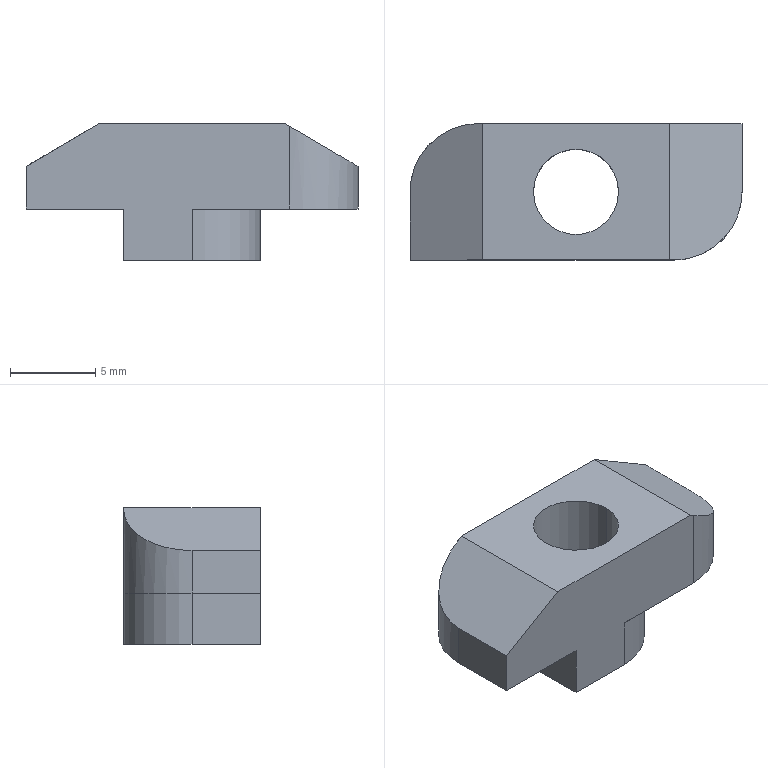Part | NX | features BREP 1 | 1 solid | 18 faces | box 19.5 x 8 x 8 mm | volume 688.541 mm3 | plane 12 | cylinder 6 | commonest cylinder face diameters 8 x4 5 x2
STEP:
#1=CARTESIAN_POINT('',(-2.5,0.,-8.));
#2=VERTEX_POINT('',#1);
#3=CARTESIAN_POINT('',(2.5,0.,-8.));
#4=VERTEX_POINT('',#3);
#5=CARTESIAN_POINT('',(0.,0.,-8.));
#6=DIRECTION('',(0.,0.,-1.));
#7=DIRECTION('',(-1.,0.,0.));
#8=AXIS2_PLACEMENT_3D('',#5,#6,#7);
#9=CIRCLE('',#8,2.5);
#10=EDGE_CURVE('',#2,#4,#9,.T.);
#11=ORIENTED_EDGE('',*,*,#10,.T.);
#12=CARTESIAN_POINT('',(2.5,0.,0.));
#13=VERTEX_POINT('',#12);
#14=CARTESIAN_POINT('',(2.5,0.,0.));
#15=DIRECTION('',(0.,0.,1.));
#16=VECTOR('',#15,1000.);
#17=LINE('',#14,#16);
#18=EDGE_CURVE('',#4,#13,#17,.T.);
#19=ORIENTED_EDGE('',*,*,#18,.T.);
#20=CARTESIAN_POINT('',(-2.5,0.,0.));
#21=VERTEX_POINT('',#20);
#22=CARTESIAN_POINT('',(0.,0.,0.));
#23=DIRECTION('',(0.,0.,-1.));
#24=DIRECTION('',(-1.,0.,0.));
#25=AXIS2_PLACEMENT_3D('',#22,#23,#24);
#26=CIRCLE('',#25,2.5);
#27=EDGE_CURVE('',#21,#13,#26,.T.);
#28=ORIENTED_EDGE('',*,*,#27,.F.);
#29=CARTESIAN_POINT('',(-2.5,0.,0.));
#30=DIRECTION('',(0.,0.,1.));
#31=VECTOR('',#30,1000.);
#32=LINE('',#29,#31);
#33=EDGE_CURVE('',#2,#21,#32,.T.);
#34=ORIENTED_EDGE('',*,*,#33,.F.);
#35=EDGE_LOOP('',(#11,#19,#28,#34));
#36=FACE_BOUND('',#35,.T.);
#37=CARTESIAN_POINT('',(0.,0.,0.));
#38=DIRECTION('',(0.,0.,1.));
#39=DIRECTION('',(-1.,0.,0.));
#40=AXIS2_PLACEMENT_3D('',#37,#38,#39);
#41=CYLINDRICAL_SURFACE('',#40,2.5);
#42=ADVANCED_FACE('',(#36),#41,.F.);
#43=CARTESIAN_POINT('',(0.,-4.,-5.));
#44=VERTEX_POINT('',#43);
#45=CARTESIAN_POINT('',(5.75,-4.,-5.));
#46=VERTEX_POINT('',#45);
#47=CARTESIAN_POINT('',(-9.75,-4.,-5.));
#48=DIRECTION('',(1.,0.,0.));
#49=VECTOR('',#48,1000.);
#50=LINE('',#47,#49);
#51=EDGE_CURVE('',#44,#46,#50,.T.);
#52=ORIENTED_EDGE('',*,*,#51,.F.);
#53=CARTESIAN_POINT('',(4.,0.,-5.));
#54=VERTEX_POINT('',#53);
#55=CARTESIAN_POINT('',(0.,0.,-5.));
#56=DIRECTION('',(0.,0.,-1.));
#57=DIRECTION('',(1.,0.,0.));
#58=AXIS2_PLACEMENT_3D('',#55,#56,#57);
#59=CIRCLE('',#58,4.);
#60=EDGE_CURVE('',#54,#44,#59,.T.);
#61=ORIENTED_EDGE('',*,*,#60,.F.);
#62=CARTESIAN_POINT('',(4.,4.,-5.));
#63=VERTEX_POINT('',#62);
#64=CARTESIAN_POINT('',(4.,-4.,-5.));
#65=DIRECTION('',(0.,1.,0.));
#66=VECTOR('',#65,1000.);
#67=LINE('',#64,#66);
#68=EDGE_CURVE('',#54,#63,#67,.T.);
#69=ORIENTED_EDGE('',*,*,#68,.T.);
#70=CARTESIAN_POINT('',(9.75,4.,-5.));
#71=VERTEX_POINT('',#70);
#72=CARTESIAN_POINT('',(-9.75,4.,-5.));
#73=DIRECTION('',(-1.,0.,0.));
#74=VECTOR('',#73,1000.);
#75=LINE('',#72,#74);
#76=EDGE_CURVE('',#71,#63,#75,.T.);
#77=ORIENTED_EDGE('',*,*,#76,.F.);
#78=CARTESIAN_POINT('',(9.75,0.,-5.));
#79=VERTEX_POINT('',#78);
#80=CARTESIAN_POINT('',(9.75,4.,-5.));
#81=DIRECTION('',(0.,1.,0.));
#82=VECTOR('',#81,1000.);
#83=LINE('',#80,#82);
#84=EDGE_CURVE('',#79,#71,#83,.T.);
#85=ORIENTED_EDGE('',*,*,#84,.F.);
#86=CARTESIAN_POINT('',(5.75,0.,-5.));
#87=DIRECTION('',(0.,0.,1.));
#88=DIRECTION('',(1.,0.,0.));
#89=AXIS2_PLACEMENT_3D('',#86,#87,#88);
#90=CIRCLE('',#89,4.);
#91=EDGE_CURVE('',#46,#79,#90,.T.);
#92=ORIENTED_EDGE('',*,*,#91,.F.);
#93=EDGE_LOOP('',(#52,#61,#69,#77,#85,#92));
#94=FACE_BOUND('',#93,.T.);
#95=CARTESIAN_POINT('',(0.,0.,-5.));
#96=DIRECTION('',(0.,0.,-1.));
#97=DIRECTION('',(0.,-1.,0.));
#98=AXIS2_PLACEMENT_3D('',#95,#96,#97);
#99=PLANE('',#98);
#100=ADVANCED_FACE('',(#94),#99,.T.);
#101=ORIENTED_EDGE('',*,*,#84,.T.);
#102=CARTESIAN_POINT('',(9.75,4.,-2.5));
#103=VERTEX_POINT('',#102);
#104=CARTESIAN_POINT('',(9.75,4.,-5.));
#105=DIRECTION('',(0.,0.,1.));
#106=VECTOR('',#105,1000.);
#107=LINE('',#104,#106);
#108=EDGE_CURVE('',#71,#103,#107,.T.);
#109=ORIENTED_EDGE('',*,*,#108,.T.);
#110=CARTESIAN_POINT('',(9.75,0.,-2.5));
#111=VERTEX_POINT('',#110);
#112=CARTESIAN_POINT('',(9.75,4.,-2.5));
#113=DIRECTION('',(0.,1.,0.));
#114=VECTOR('',#113,1000.);
#115=LINE('',#112,#114);
#116=EDGE_CURVE('',#111,#103,#115,.T.);
#117=ORIENTED_EDGE('',*,*,#116,.F.);
#118=CARTESIAN_POINT('',(9.75,0.,-5.));
#119=DIRECTION('',(0.,0.,1.));
#120=VECTOR('',#119,1000.);
#121=LINE('',#118,#120);
#122=EDGE_CURVE('',#79,#111,#121,.T.);
#123=ORIENTED_EDGE('',*,*,#122,.F.);
#124=EDGE_LOOP('',(#101,#109,#117,#123));
#125=FACE_BOUND('',#124,.T.);
#126=CARTESIAN_POINT('',(9.75,4.,-5.));
#127=DIRECTION('',(-1.,0.,0.));
#128=DIRECTION('',(0.,0.,1.));
#129=AXIS2_PLACEMENT_3D('',#126,#127,#128);
#130=PLANE('',#129);
#131=ADVANCED_FACE('',(#125),#130,.F.);
#132=CARTESIAN_POINT('',(-5.5,4.,0.));
#133=VERTEX_POINT('',#132);
#134=CARTESIAN_POINT('',(-5.75,4.,-0.1471));
#135=VERTEX_POINT('',#134);
#136=CARTESIAN_POINT('',(-9.75,4.,-2.5));
#137=DIRECTION('',(-0.8619,0.,-0.507));
#138=VECTOR('',#137,1000.);
#139=LINE('',#136,#138);
#140=EDGE_CURVE('',#133,#135,#139,.T.);
#141=ORIENTED_EDGE('',*,*,#140,.F.);
#142=CARTESIAN_POINT('',(5.5,4.,0.));
#143=VERTEX_POINT('',#142);
#144=CARTESIAN_POINT('',(-9.75,4.,0.));
#145=DIRECTION('',(-1.,0.,0.));
#146=VECTOR('',#145,1000.);
#147=LINE('',#144,#146);
#148=EDGE_CURVE('',#143,#133,#147,.T.);
#149=ORIENTED_EDGE('',*,*,#148,.F.);
#150=CARTESIAN_POINT('',(9.75,4.,-2.5));
#151=DIRECTION('',(-0.8619,0.,0.507));
#152=VECTOR('',#151,1000.);
#153=LINE('',#150,#152);
#154=EDGE_CURVE('',#103,#143,#153,.T.);
#155=ORIENTED_EDGE('',*,*,#154,.F.);
#156=ORIENTED_EDGE('',*,*,#108,.F.);
#157=ORIENTED_EDGE('',*,*,#76,.T.);
#158=CARTESIAN_POINT('',(4.,4.,-8.));
#159=VERTEX_POINT('',#158);
#160=CARTESIAN_POINT('',(4.,4.,-8.));
#161=DIRECTION('',(0.,0.,1.));
#162=VECTOR('',#161,1000.);
#163=LINE('',#160,#162);
#164=EDGE_CURVE('',#159,#63,#163,.T.);
#165=ORIENTED_EDGE('',*,*,#164,.F.);
#166=CARTESIAN_POINT('',(0.,4.,-8.));
#167=VERTEX_POINT('',#166);
#168=CARTESIAN_POINT('',(-4.,4.,-8.));
#169=DIRECTION('',(-1.,0.,0.));
#170=VECTOR('',#169,1000.);
#171=LINE('',#168,#170);
#172=EDGE_CURVE('',#159,#167,#171,.T.);
#173=ORIENTED_EDGE('',*,*,#172,.T.);
#174=CARTESIAN_POINT('',(0.,4.,-5.));
#175=VERTEX_POINT('',#174);
#176=CARTESIAN_POINT('',(0.,4.,-5.));
#177=DIRECTION('',(0.,0.,-1.));
#178=VECTOR('',#177,1000.);
#179=LINE('',#176,#178);
#180=EDGE_CURVE('',#175,#167,#179,.T.);
#181=ORIENTED_EDGE('',*,*,#180,.F.);
#182=CARTESIAN_POINT('',(-5.75,4.,-5.));
#183=VERTEX_POINT('',#182);
#184=CARTESIAN_POINT('',(-9.75,4.,-5.));
#185=DIRECTION('',(-1.,0.,0.));
#186=VECTOR('',#185,1000.);
#187=LINE('',#184,#186);
#188=EDGE_CURVE('',#175,#183,#187,.T.);
#189=ORIENTED_EDGE('',*,*,#188,.T.);
#190=CARTESIAN_POINT('',(-5.75,4.,-5.));
#191=DIRECTION('',(0.,0.,-1.));
#192=VECTOR('',#191,1000.);
#193=LINE('',#190,#192);
#194=EDGE_CURVE('',#135,#183,#193,.T.);
#195=ORIENTED_EDGE('',*,*,#194,.F.);
#196=EDGE_LOOP('',(#141,#149,#155,#156,#157,#165,#173,#181,#189,#195));
#197=FACE_BOUND('',#196,.T.);
#198=CARTESIAN_POINT('',(-9.75,4.,-5.));
#199=DIRECTION('',(0.,-1.,0.));
#200=DIRECTION('',(0.,0.,-1.));
#201=AXIS2_PLACEMENT_3D('',#198,#199,#200);
#202=PLANE('',#201);
#203=ADVANCED_FACE('',(#197),#202,.F.);
#204=CARTESIAN_POINT('',(-9.75,0.,-5.));
#205=VERTEX_POINT('',#204);
#206=CARTESIAN_POINT('',(-9.75,-4.,-5.));
#207=VERTEX_POINT('',#206);
#208=CARTESIAN_POINT('',(-9.75,4.,-5.));
#209=DIRECTION('',(0.,-1.,0.));
#210=VECTOR('',#209,1000.);
#211=LINE('',#208,#210);
#212=EDGE_CURVE('',#205,#207,#211,.T.);
#213=ORIENTED_EDGE('',*,*,#212,.T.);
#214=CARTESIAN_POINT('',(-9.75,-4.,-2.5));
#215=VERTEX_POINT('',#214);
#216=CARTESIAN_POINT('',(-9.75,-4.,-5.));
#217=DIRECTION('',(0.,0.,1.));
#218=VECTOR('',#217,1000.);
#219=LINE('',#216,#218);
#220=EDGE_CURVE('',#207,#215,#219,.T.);
#221=ORIENTED_EDGE('',*,*,#220,.T.);
#222=CARTESIAN_POINT('',(-9.75,0.,-2.5));
#223=VERTEX_POINT('',#222);
#224=CARTESIAN_POINT('',(-9.75,4.,-2.5));
#225=DIRECTION('',(0.,-1.,0.));
#226=VECTOR('',#225,1000.);
#227=LINE('',#224,#226);
#228=EDGE_CURVE('',#223,#215,#227,.T.);
#229=ORIENTED_EDGE('',*,*,#228,.F.);
#230=CARTESIAN_POINT('',(-9.75,0.,-5.));
#231=DIRECTION('',(0.,0.,1.));
#232=VECTOR('',#231,1000.);
#233=LINE('',#230,#232);
#234=EDGE_CURVE('',#205,#223,#233,.T.);
#235=ORIENTED_EDGE('',*,*,#234,.F.);
#236=EDGE_LOOP('',(#213,#221,#229,#235));
#237=FACE_BOUND('',#236,.T.);
#238=CARTESIAN_POINT('',(-9.75,4.,-5.));
#239=DIRECTION('',(1.,0.,0.));
#240=DIRECTION('',(0.,1.,0.));
#241=AXIS2_PLACEMENT_3D('',#238,#239,#240);
#242=PLANE('',#241);
#243=ADVANCED_FACE('',(#237),#242,.F.);
#244=CARTESIAN_POINT('',(5.5,-4.,0.));
#245=VERTEX_POINT('',#244);
#246=CARTESIAN_POINT('',(5.75,-4.,-0.1471));
#247=VERTEX_POINT('',#246);
#248=CARTESIAN_POINT('',(9.75,-4.,-2.5));
#249=DIRECTION('',(0.8619,0.,-0.507));
#250=VECTOR('',#249,1000.);
#251=LINE('',#248,#250);
#252=EDGE_CURVE('',#245,#247,#251,.T.);
#253=ORIENTED_EDGE('',*,*,#252,.F.);
#254=CARTESIAN_POINT('',(-5.5,-4.,0.));
#255=VERTEX_POINT('',#254);
#256=CARTESIAN_POINT('',(-9.75,-4.,0.));
#257=DIRECTION('',(1.,0.,0.));
#258=VECTOR('',#257,1000.);
#259=LINE('',#256,#258);
#260=EDGE_CURVE('',#255,#245,#259,.T.);
#261=ORIENTED_EDGE('',*,*,#260,.F.);
#262=CARTESIAN_POINT('',(-9.75,-4.,-2.5));
#263=DIRECTION('',(0.8619,0.,0.507));
#264=VECTOR('',#263,1000.);
#265=LINE('',#262,#264);
#266=EDGE_CURVE('',#215,#255,#265,.T.);
#267=ORIENTED_EDGE('',*,*,#266,.F.);
#268=ORIENTED_EDGE('',*,*,#220,.F.);
#269=CARTESIAN_POINT('',(-4.,-4.,-5.));
#270=VERTEX_POINT('',#269);
#271=CARTESIAN_POINT('',(-9.75,-4.,-5.));
#272=DIRECTION('',(1.,0.,0.));
#273=VECTOR('',#272,1000.);
#274=LINE('',#271,#273);
#275=EDGE_CURVE('',#207,#270,#274,.T.);
#276=ORIENTED_EDGE('',*,*,#275,.T.);
#277=CARTESIAN_POINT('',(-4.,-4.,-8.));
#278=VERTEX_POINT('',#277);
#279=CARTESIAN_POINT('',(-4.,-4.,-8.));
#280=DIRECTION('',(0.,0.,1.));
#281=VECTOR('',#280,1000.);
#282=LINE('',#279,#281);
#283=EDGE_CURVE('',#278,#270,#282,.T.);
#284=ORIENTED_EDGE('',*,*,#283,.F.);
#285=CARTESIAN_POINT('',(0.,-4.,-8.));
#286=VERTEX_POINT('',#285);
#287=CARTESIAN_POINT('',(-4.,-4.,-8.));
#288=DIRECTION('',(1.,0.,0.));
#289=VECTOR('',#288,1000.);
#290=LINE('',#287,#289);
#291=EDGE_CURVE('',#278,#286,#290,.T.);
#292=ORIENTED_EDGE('',*,*,#291,.T.);
#293=CARTESIAN_POINT('',(0.,-4.,-5.));
#294=DIRECTION('',(0.,0.,-1.));
#295=VECTOR('',#294,1000.);
#296=LINE('',#293,#295);
#297=EDGE_CURVE('',#44,#286,#296,.T.);
#298=ORIENTED_EDGE('',*,*,#297,.F.);
#299=ORIENTED_EDGE('',*,*,#51,.T.);
#300=CARTESIAN_POINT('',(5.75,-4.,-5.));
#301=DIRECTION('',(0.,0.,-1.));
#302=VECTOR('',#301,1000.);
#303=LINE('',#300,#302);
#304=EDGE_CURVE('',#247,#46,#303,.T.);
#305=ORIENTED_EDGE('',*,*,#304,.F.);
#306=EDGE_LOOP('',(#253,#261,#267,#268,#276,#284,#292,#298,#299,#305));
#307=FACE_BOUND('',#306,.T.);
#308=CARTESIAN_POINT('',(-9.75,-4.,-5.));
#309=DIRECTION('',(0.,1.,0.));
#310=DIRECTION('',(1.,0.,0.));
#311=AXIS2_PLACEMENT_3D('',#308,#309,#310);
#312=PLANE('',#311);
#313=ADVANCED_FACE('',(#307),#312,.F.);
#314=ORIENTED_EDGE('',*,*,#188,.F.);
#315=CARTESIAN_POINT('',(-4.,0.,-5.));
#316=VERTEX_POINT('',#315);
#317=CARTESIAN_POINT('',(0.,0.,-5.));
#318=DIRECTION('',(0.,0.,-1.));
#319=DIRECTION('',(1.,0.,0.));
#320=AXIS2_PLACEMENT_3D('',#317,#318,#319);
#321=CIRCLE('',#320,4.);
#322=EDGE_CURVE('',#316,#175,#321,.T.);
#323=ORIENTED_EDGE('',*,*,#322,.F.);
#324=CARTESIAN_POINT('',(-4.,-4.,-5.));
#325=DIRECTION('',(0.,-1.,0.));
#326=VECTOR('',#325,1000.);
#327=LINE('',#324,#326);
#328=EDGE_CURVE('',#316,#270,#327,.T.);
#329=ORIENTED_EDGE('',*,*,#328,.T.);
#330=ORIENTED_EDGE('',*,*,#275,.F.);
#331=ORIENTED_EDGE('',*,*,#212,.F.);
#332=CARTESIAN_POINT('',(-5.75,0.,-5.));
#333=DIRECTION('',(0.,0.,1.));
#334=DIRECTION('',(1.,0.,0.));
#335=AXIS2_PLACEMENT_3D('',#332,#333,#334);
#336=CIRCLE('',#335,4.);
#337=EDGE_CURVE('',#183,#205,#336,.T.);
#338=ORIENTED_EDGE('',*,*,#337,.F.);
#339=EDGE_LOOP('',(#314,#323,#329,#330,#331,#338));
#340=FACE_BOUND('',#339,.T.);
#341=CARTESIAN_POINT('',(0.,0.,-5.));
#342=DIRECTION('',(0.,0.,-1.));
#343=DIRECTION('',(0.,-1.,0.));
#344=AXIS2_PLACEMENT_3D('',#341,#342,#343);
#345=PLANE('',#344);
#346=ADVANCED_FACE('',(#340),#345,.T.);
#347=ORIENTED_EDGE('',*,*,#148,.T.);
#348=CARTESIAN_POINT('',(-5.5,0.,0.));
#349=DIRECTION('',(0.,1.,0.));
#350=VECTOR('',#349,1000.);
#351=LINE('',#348,#350);
#352=EDGE_CURVE('',#255,#133,#351,.T.);
#353=ORIENTED_EDGE('',*,*,#352,.F.);
#354=ORIENTED_EDGE('',*,*,#260,.T.);
#355=CARTESIAN_POINT('',(5.5,0.,0.));
#356=DIRECTION('',(0.,-1.,0.));
#357=VECTOR('',#356,1000.);
#358=LINE('',#355,#357);
#359=EDGE_CURVE('',#143,#245,#358,.T.);
#360=ORIENTED_EDGE('',*,*,#359,.F.);
#361=EDGE_LOOP('',(#347,#353,#354,#360));
#362=FACE_BOUND('',#361,.T.);
#363=ORIENTED_EDGE('',*,*,#27,.T.);
#364=CARTESIAN_POINT('',(0.,0.,0.));
#365=DIRECTION('',(0.,0.,-1.));
#366=DIRECTION('',(-1.,0.,0.));
#367=AXIS2_PLACEMENT_3D('',#364,#365,#366);
#368=CIRCLE('',#367,2.5);
#369=EDGE_CURVE('',#13,#21,#368,.T.);
#370=ORIENTED_EDGE('',*,*,#369,.T.);
#371=EDGE_LOOP('',(#363,#370));
#372=FACE_BOUND('',#371,.T.);
#373=CARTESIAN_POINT('',(0.,0.,0.));
#374=DIRECTION('',(0.,0.,-1.));
#375=DIRECTION('',(0.,-1.,0.));
#376=AXIS2_PLACEMENT_3D('',#373,#374,#375);
#377=PLANE('',#376);
#378=ADVANCED_FACE('',(#362,#372),#377,.F.);
#379=CARTESIAN_POINT('',(4.,0.,-8.));
#380=VERTEX_POINT('',#379);
#381=CARTESIAN_POINT('',(4.,-4.,-8.));
#382=DIRECTION('',(0.,1.,0.));
#383=VECTOR('',#382,1000.);
#384=LINE('',#381,#383);
#385=EDGE_CURVE('',#380,#159,#384,.T.);
#386=ORIENTED_EDGE('',*,*,#385,.T.);
#387=ORIENTED_EDGE('',*,*,#164,.T.);
#388=ORIENTED_EDGE('',*,*,#68,.F.);
#389=CARTESIAN_POINT('',(4.,0.,-8.));
#390=DIRECTION('',(0.,0.,1.));
#391=VECTOR('',#390,1000.);
#392=LINE('',#389,#391);
#393=EDGE_CURVE('',#380,#54,#392,.T.);
#394=ORIENTED_EDGE('',*,*,#393,.F.);
#395=EDGE_LOOP('',(#386,#387,#388,#394));
#396=FACE_BOUND('',#395,.T.);
#397=CARTESIAN_POINT('',(4.,-4.,-8.));
#398=DIRECTION('',(-1.,0.,0.));
#399=DIRECTION('',(0.,0.,1.));
#400=AXIS2_PLACEMENT_3D('',#397,#398,#399);
#401=PLANE('',#400);
#402=ADVANCED_FACE('',(#396),#401,.F.);
#403=CARTESIAN_POINT('',(-4.,0.,-8.));
#404=VERTEX_POINT('',#403);
#405=CARTESIAN_POINT('',(-4.,-4.,-8.));
#406=DIRECTION('',(0.,-1.,0.));
#407=VECTOR('',#406,1000.);
#408=LINE('',#405,#407);
#409=EDGE_CURVE('',#404,#278,#408,.T.);
#410=ORIENTED_EDGE('',*,*,#409,.T.);
#411=ORIENTED_EDGE('',*,*,#283,.T.);
#412=ORIENTED_EDGE('',*,*,#328,.F.);
#413=CARTESIAN_POINT('',(-4.,0.,-8.));
#414=DIRECTION('',(0.,0.,1.));
#415=VECTOR('',#414,1000.);
#416=LINE('',#413,#415);
#417=EDGE_CURVE('',#404,#316,#416,.T.);
#418=ORIENTED_EDGE('',*,*,#417,.F.);
#419=EDGE_LOOP('',(#410,#411,#412,#418));
#420=FACE_BOUND('',#419,.T.);
#421=CARTESIAN_POINT('',(-4.,-4.,-8.));
#422=DIRECTION('',(1.,0.,0.));
#423=DIRECTION('',(0.,1.,0.));
#424=AXIS2_PLACEMENT_3D('',#421,#422,#423);
#425=PLANE('',#424);
#426=ADVANCED_FACE('',(#420),#425,.F.);
#427=ORIENTED_EDGE('',*,*,#291,.F.);
#428=ORIENTED_EDGE('',*,*,#409,.F.);
#429=CARTESIAN_POINT('',(0.,0.,-8.));
#430=DIRECTION('',(0.,0.,1.));
#431=DIRECTION('',(-1.,0.,0.));
#432=AXIS2_PLACEMENT_3D('',#429,#430,#431);
#433=CIRCLE('',#432,4.);
#434=EDGE_CURVE('',#167,#404,#433,.T.);
#435=ORIENTED_EDGE('',*,*,#434,.F.);
#436=ORIENTED_EDGE('',*,*,#172,.F.);
#437=ORIENTED_EDGE('',*,*,#385,.F.);
#438=CARTESIAN_POINT('',(0.,0.,-8.));
#439=DIRECTION('',(0.,0.,1.));
#440=DIRECTION('',(-1.,0.,0.));
#441=AXIS2_PLACEMENT_3D('',#438,#439,#440);
#442=CIRCLE('',#441,4.);
#443=EDGE_CURVE('',#286,#380,#442,.T.);
#444=ORIENTED_EDGE('',*,*,#443,.F.);
#445=EDGE_LOOP('',(#427,#428,#435,#436,#437,#444));
#446=FACE_BOUND('',#445,.T.);
#447=ORIENTED_EDGE('',*,*,#10,.F.);
#448=CARTESIAN_POINT('',(0.,0.,-8.));
#449=DIRECTION('',(0.,0.,-1.));
#450=DIRECTION('',(-1.,0.,0.));
#451=AXIS2_PLACEMENT_3D('',#448,#449,#450);
#452=CIRCLE('',#451,2.5);
#453=EDGE_CURVE('',#4,#2,#452,.T.);
#454=ORIENTED_EDGE('',*,*,#453,.F.);
#455=EDGE_LOOP('',(#447,#454));
#456=FACE_BOUND('',#455,.T.);
#457=CARTESIAN_POINT('',(0.,0.,-8.));
#458=DIRECTION('',(0.,0.,1.));
#459=DIRECTION('',(1.,0.,0.));
#460=AXIS2_PLACEMENT_3D('',#457,#458,#459);
#461=PLANE('',#460);
#462=ADVANCED_FACE('',(#446,#456),#461,.F.);
#463=ORIENTED_EDGE('',*,*,#18,.F.);
#464=ORIENTED_EDGE('',*,*,#453,.T.);
#465=ORIENTED_EDGE('',*,*,#33,.T.);
#466=ORIENTED_EDGE('',*,*,#369,.F.);
#467=EDGE_LOOP('',(#463,#464,#465,#466));
#468=FACE_BOUND('',#467,.T.);
#469=CARTESIAN_POINT('',(0.,0.,0.));
#470=DIRECTION('',(0.,0.,1.));
#471=DIRECTION('',(-1.,0.,0.));
#472=AXIS2_PLACEMENT_3D('',#469,#470,#471);
#473=CYLINDRICAL_SURFACE('',#472,2.5);
#474=ADVANCED_FACE('',(#468),#473,.F.);
#475=ORIENTED_EDGE('',*,*,#116,.T.);
#476=ORIENTED_EDGE('',*,*,#154,.T.);
#477=ORIENTED_EDGE('',*,*,#359,.T.);
#478=ORIENTED_EDGE('',*,*,#252,.T.);
#479=CARTESIAN_POINT('',(9.75,0.,-2.5));
#480=CARTESIAN_POINT('',(9.75,-2.343,-2.5));
#481=CARTESIAN_POINT('',(8.093,-4.,-1.525));
#482=CARTESIAN_POINT('',(5.75,-4.,-0.1471));
#483=(BOUNDED_CURVE()B_SPLINE_CURVE(3,(#479,#480,#481,#482),.UNSPECIFIED.,.F.,.F.)B_SPLINE_CURVE_WITH_KNOTS((4,4),(3.142,4.712),.UNSPECIFIED.)CURVE()GEOMETRIC_REPRESENTATION_ITEM()RATIONAL_B_SPLINE_CURVE((1.,0.8047,0.8047,1.))REPRESENTATION_ITEM(''));
#484=EDGE_CURVE('',#111,#247,#483,.T.);
#485=ORIENTED_EDGE('',*,*,#484,.F.);
#486=EDGE_LOOP('',(#475,#476,#477,#478,#485));
#487=FACE_BOUND('',#486,.T.);
#488=CARTESIAN_POINT('',(9.75,4.,-2.5));
#489=DIRECTION('',(-0.507,0.,-0.8619));
#490=DIRECTION('',(-0.8619,0.,0.507));
#491=AXIS2_PLACEMENT_3D('',#488,#489,#490);
#492=PLANE('',#491);
#493=ADVANCED_FACE('',(#487),#492,.F.);
#494=ORIENTED_EDGE('',*,*,#228,.T.);
#495=ORIENTED_EDGE('',*,*,#266,.T.);
#496=ORIENTED_EDGE('',*,*,#352,.T.);
#497=ORIENTED_EDGE('',*,*,#140,.T.);
#498=CARTESIAN_POINT('',(-9.75,0.,-2.5));
#499=CARTESIAN_POINT('',(-9.75,2.343,-2.5));
#500=CARTESIAN_POINT('',(-8.093,4.,-1.525));
#501=CARTESIAN_POINT('',(-5.75,4.,-0.1471));
#502=(BOUNDED_CURVE()B_SPLINE_CURVE(3,(#498,#499,#500,#501),.UNSPECIFIED.,.F.,.F.)B_SPLINE_CURVE_WITH_KNOTS((4,4),(3.142,4.712),.UNSPECIFIED.)CURVE()GEOMETRIC_REPRESENTATION_ITEM()RATIONAL_B_SPLINE_CURVE((1.,0.8047,0.8047,1.))REPRESENTATION_ITEM(''));
#503=EDGE_CURVE('',#223,#135,#502,.T.);
#504=ORIENTED_EDGE('',*,*,#503,.F.);
#505=EDGE_LOOP('',(#494,#495,#496,#497,#504));
#506=FACE_BOUND('',#505,.T.);
#507=CARTESIAN_POINT('',(-9.75,4.,-2.5));
#508=DIRECTION('',(0.507,0.,-0.8619));
#509=DIRECTION('',(0.,-1.,0.));
#510=AXIS2_PLACEMENT_3D('',#507,#508,#509);
#511=PLANE('',#510);
#512=ADVANCED_FACE('',(#506),#511,.F.);
#513=ORIENTED_EDGE('',*,*,#91,.T.);
#514=ORIENTED_EDGE('',*,*,#122,.T.);
#515=ORIENTED_EDGE('',*,*,#484,.T.);
#516=ORIENTED_EDGE('',*,*,#304,.T.);
#517=EDGE_LOOP('',(#513,#514,#515,#516));
#518=FACE_BOUND('',#517,.T.);
#519=CARTESIAN_POINT('',(5.75,0.,-5.));
#520=DIRECTION('',(0.,0.,1.));
#521=DIRECTION('',(-1.,0.,0.));
#522=AXIS2_PLACEMENT_3D('',#519,#520,#521);
#523=CYLINDRICAL_SURFACE('',#522,4.);
#524=ADVANCED_FACE('',(#518),#523,.T.);
#525=ORIENTED_EDGE('',*,*,#337,.T.);
#526=ORIENTED_EDGE('',*,*,#234,.T.);
#527=ORIENTED_EDGE('',*,*,#503,.T.);
#528=ORIENTED_EDGE('',*,*,#194,.T.);
#529=EDGE_LOOP('',(#525,#526,#527,#528));
#530=FACE_BOUND('',#529,.T.);
#531=CARTESIAN_POINT('',(-5.75,0.,-5.));
#532=DIRECTION('',(0.,0.,1.));
#533=DIRECTION('',(-1.,0.,0.));
#534=AXIS2_PLACEMENT_3D('',#531,#532,#533);
#535=CYLINDRICAL_SURFACE('',#534,4.);
#536=ADVANCED_FACE('',(#530),#535,.T.);
#537=ORIENTED_EDGE('',*,*,#443,.T.);
#538=ORIENTED_EDGE('',*,*,#393,.T.);
#539=ORIENTED_EDGE('',*,*,#60,.T.);
#540=ORIENTED_EDGE('',*,*,#297,.T.);
#541=EDGE_LOOP('',(#537,#538,#539,#540));
#542=FACE_BOUND('',#541,.T.);
#543=CARTESIAN_POINT('',(0.,0.,-8.));
#544=DIRECTION('',(0.,0.,1.));
#545=DIRECTION('',(-1.,0.,0.));
#546=AXIS2_PLACEMENT_3D('',#543,#544,#545);
#547=CYLINDRICAL_SURFACE('',#546,4.);
#548=ADVANCED_FACE('',(#542),#547,.T.);
#549=ORIENTED_EDGE('',*,*,#434,.T.);
#550=ORIENTED_EDGE('',*,*,#417,.T.);
#551=ORIENTED_EDGE('',*,*,#322,.T.);
#552=ORIENTED_EDGE('',*,*,#180,.T.);
#553=EDGE_LOOP('',(#549,#550,#551,#552));
#554=FACE_BOUND('',#553,.T.);
#555=CARTESIAN_POINT('',(0.,0.,-8.));
#556=DIRECTION('',(0.,0.,1.));
#557=DIRECTION('',(-1.,0.,0.));
#558=AXIS2_PLACEMENT_3D('',#555,#556,#557);
#559=CYLINDRICAL_SURFACE('',#558,4.);
#560=ADVANCED_FACE('',(#554),#559,.T.);
#561=CLOSED_SHELL('',(#42,#100,#131,#203,#243,#313,#346,#378,#402,#426,#462,#474,#493,#512,#524,#536,#548,#560));
#562=MANIFOLD_SOLID_BREP('',#561);
#563=(LENGTH_UNIT()NAMED_UNIT(*)SI_UNIT(.MILLI.,.METRE.));
#564=UNCERTAINTY_MEASURE_WITH_UNIT(LENGTH_MEASURE(0.00001),#563,'','');
#565=(NAMED_UNIT(*)PLANE_ANGLE_UNIT()SI_UNIT($,.RADIAN.));
#566=(NAMED_UNIT(*)SI_UNIT($,.STERADIAN.)SOLID_ANGLE_UNIT());
#567=(GEOMETRIC_REPRESENTATION_CONTEXT(3)GLOBAL_UNCERTAINTY_ASSIGNED_CONTEXT((#564))GLOBAL_UNIT_ASSIGNED_CONTEXT((#563,#565,#566))REPRESENTATION_CONTEXT('',''));
#568=ADVANCED_BREP_SHAPE_REPRESENTATION('',(#562),#567);